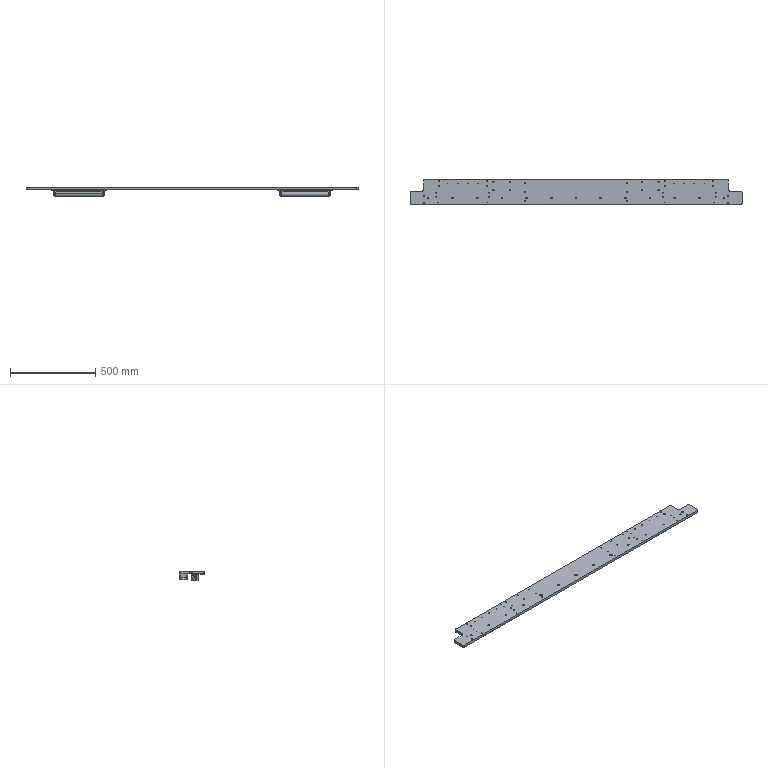Part | SolidWorks | features ReferencePattern 5, LocalLPattern 2, MirrorCompFeat 1 | 15 solids | 475 faces | box 1950 x 150 x 55.5 mm | volume 5101027 mm3 | cylinder 280 | plane 179 | cone 16 | commonest cylinder face diameters 6.8 x60 9 x42 5 x40 7 x40 15 x36 11 x16